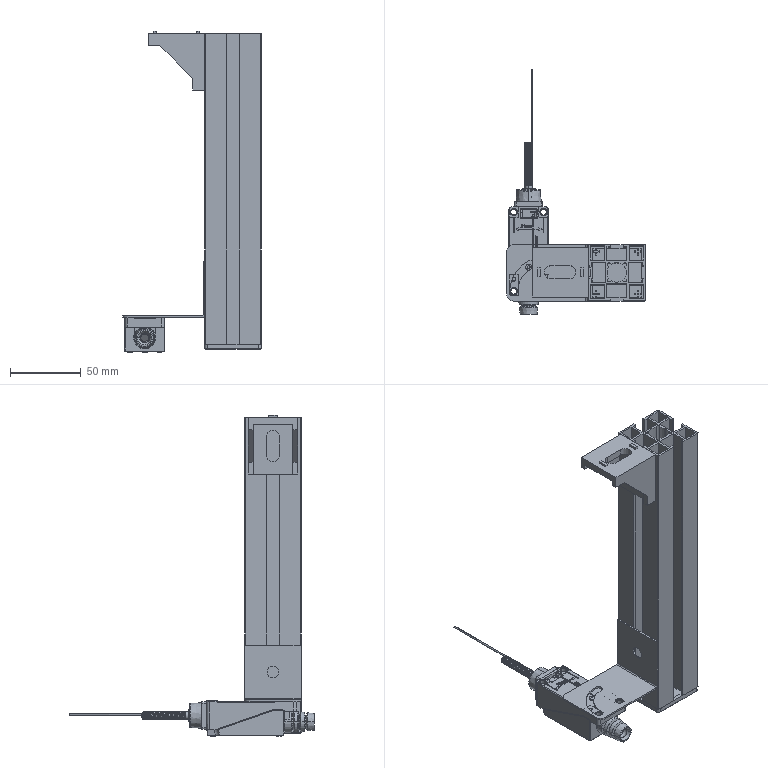Part | 4 solids | 1207 faces | box 98 x 173.5 x 227.42 mm | volume 142865 mm3 | plane 553 | cylinder 270 | spline 162 | cone 119 | torus 89 | sphere 14 | commonest cylinder face diameters 1 x53 3 x18 0.6 x16 1.5 x16 2.5 x16 1.56 x12